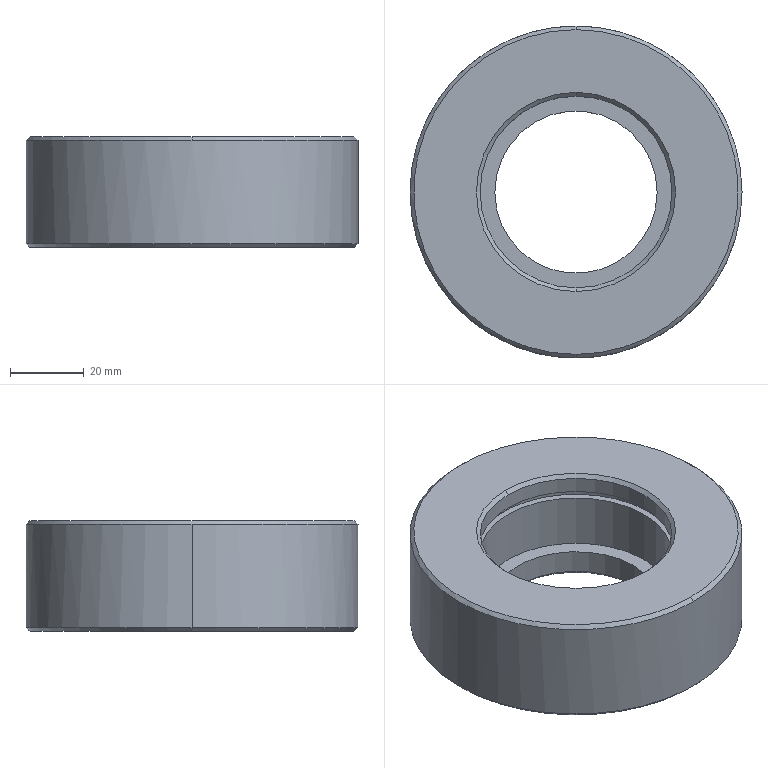Part | STEP file | 1 solid | 23 faces | box 90 x 90 x 30 mm | volume 130580 mm3 | cylinder 10 | cone 8 | plane 5 | commonest cylinder face diameters 52 x4 44 x2 55.5 x2 90 x2